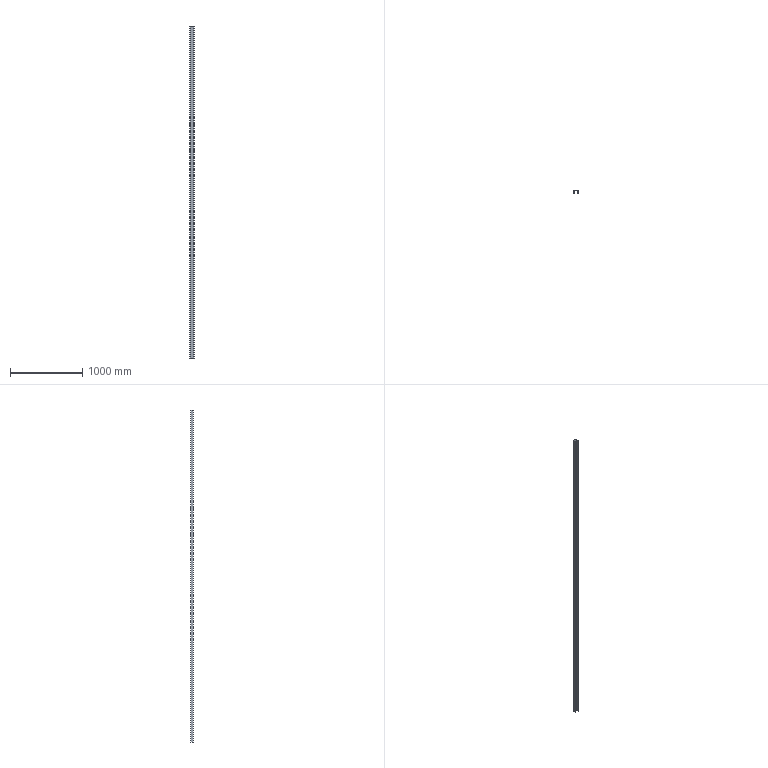Part | SolidWorks | features FlatPattern 1, SMBaseFlange 1, SheetMetal 1 | 1 solid | 22 faces | box 57 x 40 x 4600 mm | volume 1199908 mm3 | plane 18 | cylinder 4 | commonest cylinder face diameters 4 x2 8 x2
STEP:
#1=CARTESIAN_POINT('',(4.,0.,2300.));
#2=VERTEX_POINT('',#1);
#3=CARTESIAN_POINT('',(4.,-2.,2300.));
#4=VERTEX_POINT('',#3);
#5=CARTESIAN_POINT('',(4.,0.,2300.));
#6=DIRECTION('',(0.,-1.,0.));
#7=VECTOR('',#6,1000.);
#8=LINE('',#5,#7);
#9=EDGE_CURVE('',#2,#4,#8,.T.);
#10=ORIENTED_EDGE('',*,*,#9,.F.);
#11=CARTESIAN_POINT('',(0.,-4.,2300.));
#12=VERTEX_POINT('',#11);
#13=CARTESIAN_POINT('',(4.,-4.,2300.));
#14=DIRECTION('',(0.,0.,-1.));
#15=DIRECTION('',(1.,0.,0.));
#16=AXIS2_PLACEMENT_3D('',#13,#14,#15);
#17=CIRCLE('',#16,4.);
#18=EDGE_CURVE('',#12,#2,#17,.T.);
#19=ORIENTED_EDGE('',*,*,#18,.F.);
#20=CARTESIAN_POINT('',(2.,-4.,2300.));
#21=VERTEX_POINT('',#20);
#22=CARTESIAN_POINT('',(2.,-4.,2300.));
#23=DIRECTION('',(-1.,0.,0.));
#24=VECTOR('',#23,1000.);
#25=LINE('',#22,#24);
#26=EDGE_CURVE('',#21,#12,#25,.T.);
#27=ORIENTED_EDGE('',*,*,#26,.F.);
#28=CARTESIAN_POINT('',(4.,-4.,2300.));
#29=DIRECTION('',(0.,0.,-1.));
#30=DIRECTION('',(1.,0.,0.));
#31=AXIS2_PLACEMENT_3D('',#28,#29,#30);
#32=CIRCLE('',#31,2.);
#33=EDGE_CURVE('',#21,#4,#32,.T.);
#34=ORIENTED_EDGE('',*,*,#33,.T.);
#35=EDGE_LOOP('',(#10,#19,#27,#34));
#36=FACE_OUTER_BOUND('',#35,.T.);
#37=CARTESIAN_POINT('',(4.,0.,2300.));
#38=DIRECTION('',(0.,0.,1.));
#39=DIRECTION('',(1.,0.,0.));
#40=AXIS2_PLACEMENT_3D('',#37,#38,#39);
#41=PLANE('',#40);
#42=ADVANCED_FACE('',(#36),#41,.T.);
#43=CARTESIAN_POINT('',(53.,0.,2300.));
#44=VERTEX_POINT('',#43);
#45=CARTESIAN_POINT('',(57.,0.,2300.));
#46=DIRECTION('',(1.,0.,0.));
#47=VECTOR('',#46,1000.);
#48=LINE('',#45,#47);
#49=EDGE_CURVE('',#2,#44,#48,.T.);
#50=ORIENTED_EDGE('',*,*,#49,.F.);
#51=ORIENTED_EDGE('',*,*,#9,.T.);
#52=CARTESIAN_POINT('',(53.,-2.,2300.));
#53=VERTEX_POINT('',#52);
#54=CARTESIAN_POINT('',(57.,-2.,2300.));
#55=DIRECTION('',(1.,0.,0.));
#56=VECTOR('',#55,1000.);
#57=LINE('',#54,#56);
#58=EDGE_CURVE('',#4,#53,#57,.T.);
#59=ORIENTED_EDGE('',*,*,#58,.T.);
#60=CARTESIAN_POINT('',(53.,-2.,2300.));
#61=DIRECTION('',(0.,1.,0.));
#62=VECTOR('',#61,1000.);
#63=LINE('',#60,#62);
#64=EDGE_CURVE('',#53,#44,#63,.T.);
#65=ORIENTED_EDGE('',*,*,#64,.T.);
#66=EDGE_LOOP('',(#50,#51,#59,#65));
#67=FACE_OUTER_BOUND('',#66,.T.);
#68=CARTESIAN_POINT('',(2.,-4.,2300.));
#69=DIRECTION('',(0.,0.,1.));
#70=DIRECTION('',(1.,0.,0.));
#71=AXIS2_PLACEMENT_3D('',#68,#69,#70);
#72=PLANE('',#71);
#73=ADVANCED_FACE('',(#67),#72,.T.);
#74=CARTESIAN_POINT('',(0.,-4.,-2300.));
#75=VERTEX_POINT('',#74);
#76=CARTESIAN_POINT('',(2.,-4.,-2300.));
#77=VERTEX_POINT('',#76);
#78=CARTESIAN_POINT('',(0.,-4.,-2300.));
#79=DIRECTION('',(1.,0.,0.));
#80=VECTOR('',#79,1000.);
#81=LINE('',#78,#80);
#82=EDGE_CURVE('',#75,#77,#81,.T.);
#83=ORIENTED_EDGE('',*,*,#82,.F.);
#84=CARTESIAN_POINT('',(4.,0.,-2300.));
#85=VERTEX_POINT('',#84);
#86=CARTESIAN_POINT('',(4.,-4.,-2300.));
#87=DIRECTION('',(0.,0.,-1.));
#88=DIRECTION('',(1.,0.,0.));
#89=AXIS2_PLACEMENT_3D('',#86,#87,#88);
#90=CIRCLE('',#89,4.);
#91=EDGE_CURVE('',#75,#85,#90,.T.);
#92=ORIENTED_EDGE('',*,*,#91,.T.);
#93=CARTESIAN_POINT('',(4.,-2.,-2300.));
#94=VERTEX_POINT('',#93);
#95=CARTESIAN_POINT('',(4.,-2.,-2300.));
#96=DIRECTION('',(0.,1.,0.));
#97=VECTOR('',#96,1000.);
#98=LINE('',#95,#97);
#99=EDGE_CURVE('',#94,#85,#98,.T.);
#100=ORIENTED_EDGE('',*,*,#99,.F.);
#101=CARTESIAN_POINT('',(4.,-4.,-2300.));
#102=DIRECTION('',(0.,0.,-1.));
#103=DIRECTION('',(1.,0.,0.));
#104=AXIS2_PLACEMENT_3D('',#101,#102,#103);
#105=CIRCLE('',#104,2.);
#106=EDGE_CURVE('',#77,#94,#105,.T.);
#107=ORIENTED_EDGE('',*,*,#106,.F.);
#108=EDGE_LOOP('',(#83,#92,#100,#107));
#109=FACE_OUTER_BOUND('',#108,.T.);
#110=CARTESIAN_POINT('',(0.,-4.,-2300.));
#111=DIRECTION('',(0.,0.,-1.));
#112=DIRECTION('',(-1.,0.,0.));
#113=AXIS2_PLACEMENT_3D('',#110,#111,#112);
#114=PLANE('',#113);
#115=ADVANCED_FACE('',(#109),#114,.T.);
#116=CARTESIAN_POINT('',(0.,-40.,-2300.));
#117=VERTEX_POINT('',#116);
#118=CARTESIAN_POINT('',(0.,0.,-2300.));
#119=DIRECTION('',(0.,1.,0.));
#120=VECTOR('',#119,1000.);
#121=LINE('',#118,#120);
#122=EDGE_CURVE('',#117,#75,#121,.T.);
#123=ORIENTED_EDGE('',*,*,#122,.T.);
#124=ORIENTED_EDGE('',*,*,#82,.T.);
#125=CARTESIAN_POINT('',(2.,-40.,-2300.));
#126=VERTEX_POINT('',#125);
#127=CARTESIAN_POINT('',(2.,0.,-2300.));
#128=DIRECTION('',(0.,1.,0.));
#129=VECTOR('',#128,1000.);
#130=LINE('',#127,#129);
#131=EDGE_CURVE('',#126,#77,#130,.T.);
#132=ORIENTED_EDGE('',*,*,#131,.F.);
#133=CARTESIAN_POINT('',(2.,-40.,-2300.));
#134=DIRECTION('',(-1.,0.,0.));
#135=VECTOR('',#134,1000.);
#136=LINE('',#133,#135);
#137=EDGE_CURVE('',#126,#117,#136,.T.);
#138=ORIENTED_EDGE('',*,*,#137,.T.);
#139=EDGE_LOOP('',(#123,#124,#132,#138));
#140=FACE_OUTER_BOUND('',#139,.T.);
#141=CARTESIAN_POINT('',(4.,-2.,-2300.));
#142=DIRECTION('',(0.,0.,-1.));
#143=DIRECTION('',(-1.,0.,0.));
#144=AXIS2_PLACEMENT_3D('',#141,#142,#143);
#145=PLANE('',#144);
#146=ADVANCED_FACE('',(#140),#145,.T.);
#147=CARTESIAN_POINT('',(57.,-4.,2300.));
#148=VERTEX_POINT('',#147);
#149=CARTESIAN_POINT('',(55.,-4.,2300.));
#150=VERTEX_POINT('',#149);
#151=CARTESIAN_POINT('',(57.,-4.,2300.));
#152=DIRECTION('',(-1.,0.,0.));
#153=VECTOR('',#152,1000.);
#154=LINE('',#151,#153);
#155=EDGE_CURVE('',#148,#150,#154,.T.);
#156=ORIENTED_EDGE('',*,*,#155,.F.);
#157=CARTESIAN_POINT('',(53.,-4.,2300.));
#158=DIRECTION('',(0.,0.,-1.));
#159=DIRECTION('',(1.,0.,0.));
#160=AXIS2_PLACEMENT_3D('',#157,#158,#159);
#161=CIRCLE('',#160,4.);
#162=EDGE_CURVE('',#44,#148,#161,.T.);
#163=ORIENTED_EDGE('',*,*,#162,.F.);
#164=ORIENTED_EDGE('',*,*,#64,.F.);
#165=CARTESIAN_POINT('',(53.,-4.,2300.));
#166=DIRECTION('',(0.,0.,-1.));
#167=DIRECTION('',(1.,0.,0.));
#168=AXIS2_PLACEMENT_3D('',#165,#166,#167);
#169=CIRCLE('',#168,2.);
#170=EDGE_CURVE('',#53,#150,#169,.T.);
#171=ORIENTED_EDGE('',*,*,#170,.T.);
#172=EDGE_LOOP('',(#156,#163,#164,#171));
#173=FACE_OUTER_BOUND('',#172,.T.);
#174=CARTESIAN_POINT('',(57.,-4.,2300.));
#175=DIRECTION('',(0.,0.,1.));
#176=DIRECTION('',(1.,0.,0.));
#177=AXIS2_PLACEMENT_3D('',#174,#175,#176);
#178=PLANE('',#177);
#179=ADVANCED_FACE('',(#173),#178,.T.);
#180=CARTESIAN_POINT('',(57.,-40.,2300.));
#181=VERTEX_POINT('',#180);
#182=CARTESIAN_POINT('',(57.,0.,2300.));
#183=DIRECTION('',(0.,-1.,0.));
#184=VECTOR('',#183,1000.);
#185=LINE('',#182,#184);
#186=EDGE_CURVE('',#148,#181,#185,.T.);
#187=ORIENTED_EDGE('',*,*,#186,.F.);
#188=ORIENTED_EDGE('',*,*,#155,.T.);
#189=CARTESIAN_POINT('',(55.,-40.,2300.));
#190=VERTEX_POINT('',#189);
#191=CARTESIAN_POINT('',(55.,0.,2300.));
#192=DIRECTION('',(0.,-1.,0.));
#193=VECTOR('',#192,1000.);
#194=LINE('',#191,#193);
#195=EDGE_CURVE('',#150,#190,#194,.T.);
#196=ORIENTED_EDGE('',*,*,#195,.T.);
#197=CARTESIAN_POINT('',(57.,-40.,2300.));
#198=DIRECTION('',(-1.,0.,0.));
#199=VECTOR('',#198,1000.);
#200=LINE('',#197,#199);
#201=EDGE_CURVE('',#181,#190,#200,.T.);
#202=ORIENTED_EDGE('',*,*,#201,.F.);
#203=EDGE_LOOP('',(#187,#188,#196,#202));
#204=FACE_OUTER_BOUND('',#203,.T.);
#205=CARTESIAN_POINT('',(53.,-2.,2300.));
#206=DIRECTION('',(0.,0.,1.));
#207=DIRECTION('',(1.,0.,0.));
#208=AXIS2_PLACEMENT_3D('',#205,#206,#207);
#209=PLANE('',#208);
#210=ADVANCED_FACE('',(#204),#209,.T.);
#211=CARTESIAN_POINT('',(53.,0.,-2300.));
#212=VERTEX_POINT('',#211);
#213=CARTESIAN_POINT('',(53.,-2.,-2300.));
#214=VERTEX_POINT('',#213);
#215=CARTESIAN_POINT('',(53.,0.,-2300.));
#216=DIRECTION('',(0.,-1.,0.));
#217=VECTOR('',#216,1000.);
#218=LINE('',#215,#217);
#219=EDGE_CURVE('',#212,#214,#218,.T.);
#220=ORIENTED_EDGE('',*,*,#219,.F.);
#221=CARTESIAN_POINT('',(57.,-4.,-2300.));
#222=VERTEX_POINT('',#221);
#223=CARTESIAN_POINT('',(53.,-4.,-2300.));
#224=DIRECTION('',(0.,0.,-1.));
#225=DIRECTION('',(1.,0.,0.));
#226=AXIS2_PLACEMENT_3D('',#223,#224,#225);
#227=CIRCLE('',#226,4.);
#228=EDGE_CURVE('',#212,#222,#227,.T.);
#229=ORIENTED_EDGE('',*,*,#228,.T.);
#230=CARTESIAN_POINT('',(55.,-4.,-2300.));
#231=VERTEX_POINT('',#230);
#232=CARTESIAN_POINT('',(55.,-4.,-2300.));
#233=DIRECTION('',(1.,0.,0.));
#234=VECTOR('',#233,1000.);
#235=LINE('',#232,#234);
#236=EDGE_CURVE('',#231,#222,#235,.T.);
#237=ORIENTED_EDGE('',*,*,#236,.F.);
#238=CARTESIAN_POINT('',(53.,-4.,-2300.));
#239=DIRECTION('',(0.,0.,-1.));
#240=DIRECTION('',(1.,0.,0.));
#241=AXIS2_PLACEMENT_3D('',#238,#239,#240);
#242=CIRCLE('',#241,2.);
#243=EDGE_CURVE('',#214,#231,#242,.T.);
#244=ORIENTED_EDGE('',*,*,#243,.F.);
#245=EDGE_LOOP('',(#220,#229,#237,#244));
#246=FACE_OUTER_BOUND('',#245,.T.);
#247=CARTESIAN_POINT('',(53.,0.,-2300.));
#248=DIRECTION('',(0.,0.,-1.));
#249=DIRECTION('',(-1.,0.,0.));
#250=AXIS2_PLACEMENT_3D('',#247,#248,#249);
#251=PLANE('',#250);
#252=ADVANCED_FACE('',(#246),#251,.T.);
#253=CARTESIAN_POINT('',(57.,0.,-2300.));
#254=DIRECTION('',(1.,0.,0.));
#255=VECTOR('',#254,1000.);
#256=LINE('',#253,#255);
#257=EDGE_CURVE('',#85,#212,#256,.T.);
#258=ORIENTED_EDGE('',*,*,#257,.T.);
#259=ORIENTED_EDGE('',*,*,#219,.T.);
#260=CARTESIAN_POINT('',(57.,-2.,-2300.));
#261=DIRECTION('',(1.,0.,0.));
#262=VECTOR('',#261,1000.);
#263=LINE('',#260,#262);
#264=EDGE_CURVE('',#94,#214,#263,.T.);
#265=ORIENTED_EDGE('',*,*,#264,.F.);
#266=ORIENTED_EDGE('',*,*,#99,.T.);
#267=EDGE_LOOP('',(#258,#259,#265,#266));
#268=FACE_OUTER_BOUND('',#267,.T.);
#269=CARTESIAN_POINT('',(55.,-4.,-2300.));
#270=DIRECTION('',(0.,0.,-1.));
#271=DIRECTION('',(-1.,0.,0.));
#272=AXIS2_PLACEMENT_3D('',#269,#270,#271);
#273=PLANE('',#272);
#274=ADVANCED_FACE('',(#268),#273,.T.);
#275=CARTESIAN_POINT('',(55.,-40.,-2300.));
#276=VERTEX_POINT('',#275);
#277=CARTESIAN_POINT('',(55.,0.,-2300.));
#278=DIRECTION('',(0.,-1.,0.));
#279=VECTOR('',#278,1000.);
#280=LINE('',#277,#279);
#281=EDGE_CURVE('',#231,#276,#280,.T.);
#282=ORIENTED_EDGE('',*,*,#281,.T.);
#283=CARTESIAN_POINT('',(55.,-40.,2300.));
#284=DIRECTION('',(0.,0.,-1.));
#285=VECTOR('',#284,1000.);
#286=LINE('',#283,#285);
#287=EDGE_CURVE('',#190,#276,#286,.T.);
#288=ORIENTED_EDGE('',*,*,#287,.F.);
#289=ORIENTED_EDGE('',*,*,#195,.F.);
#290=CARTESIAN_POINT('',(55.,-4.,2300.));
#291=DIRECTION('',(0.,0.,-1.));
#292=VECTOR('',#291,1000.);
#293=LINE('',#290,#292);
#294=EDGE_CURVE('',#150,#231,#293,.T.);
#295=ORIENTED_EDGE('',*,*,#294,.T.);
#296=EDGE_LOOP('',(#282,#288,#289,#295));
#297=FACE_OUTER_BOUND('',#296,.T.);
#298=CARTESIAN_POINT('',(55.,0.,2300.));
#299=DIRECTION('',(1.,0.,0.));
#300=DIRECTION('',(0.,0.,-1.));
#301=AXIS2_PLACEMENT_3D('',#298,#299,#300);
#302=PLANE('',#301);
#303=ADVANCED_FACE('',(#297),#302,.F.);
#304=CARTESIAN_POINT('',(57.,-40.,-2300.));
#305=VERTEX_POINT('',#304);
#306=CARTESIAN_POINT('',(57.,-40.,-2300.));
#307=DIRECTION('',(-1.,0.,0.));
#308=VECTOR('',#307,1000.);
#309=LINE('',#306,#308);
#310=EDGE_CURVE('',#305,#276,#309,.T.);
#311=ORIENTED_EDGE('',*,*,#310,.F.);
#312=CARTESIAN_POINT('',(57.,-40.,2300.));
#313=DIRECTION('',(0.,0.,-1.));
#314=VECTOR('',#313,1000.);
#315=LINE('',#312,#314);
#316=EDGE_CURVE('',#181,#305,#315,.T.);
#317=ORIENTED_EDGE('',*,*,#316,.F.);
#318=ORIENTED_EDGE('',*,*,#201,.T.);
#319=ORIENTED_EDGE('',*,*,#287,.T.);
#320=EDGE_LOOP('',(#311,#317,#318,#319));
#321=FACE_OUTER_BOUND('',#320,.T.);
#322=CARTESIAN_POINT('',(57.,-40.,2300.));
#323=DIRECTION('',(0.,-1.,0.));
#324=DIRECTION('',(0.,0.,-1.));
#325=AXIS2_PLACEMENT_3D('',#322,#323,#324);
#326=PLANE('',#325);
#327=ADVANCED_FACE('',(#321),#326,.T.);
#328=CARTESIAN_POINT('',(57.,0.,-2300.));
#329=DIRECTION('',(0.,-1.,0.));
#330=VECTOR('',#329,1000.);
#331=LINE('',#328,#330);
#332=EDGE_CURVE('',#222,#305,#331,.T.);
#333=ORIENTED_EDGE('',*,*,#332,.F.);
#334=CARTESIAN_POINT('',(57.,-4.,2300.));
#335=DIRECTION('',(0.,0.,-1.));
#336=VECTOR('',#335,1000.);
#337=LINE('',#334,#336);
#338=EDGE_CURVE('',#148,#222,#337,.T.);
#339=ORIENTED_EDGE('',*,*,#338,.F.);
#340=ORIENTED_EDGE('',*,*,#186,.T.);
#341=ORIENTED_EDGE('',*,*,#316,.T.);
#342=EDGE_LOOP('',(#333,#339,#340,#341));
#343=FACE_OUTER_BOUND('',#342,.T.);
#344=CARTESIAN_POINT('',(57.,0.,2300.));
#345=DIRECTION('',(1.,0.,0.));
#346=DIRECTION('',(0.,0.,-1.));
#347=AXIS2_PLACEMENT_3D('',#344,#345,#346);
#348=PLANE('',#347);
#349=ADVANCED_FACE('',(#343),#348,.T.);
#350=ORIENTED_EDGE('',*,*,#228,.F.);
#351=CARTESIAN_POINT('',(53.,0.,2300.));
#352=DIRECTION('',(0.,0.,-1.));
#353=VECTOR('',#352,1000.);
#354=LINE('',#351,#353);
#355=EDGE_CURVE('',#44,#212,#354,.T.);
#356=ORIENTED_EDGE('',*,*,#355,.F.);
#357=ORIENTED_EDGE('',*,*,#162,.T.);
#358=ORIENTED_EDGE('',*,*,#338,.T.);
#359=EDGE_LOOP('',(#350,#356,#357,#358));
#360=FACE_OUTER_BOUND('',#359,.T.);
#361=CARTESIAN_POINT('',(53.,-4.,2300.));
#362=DIRECTION('',(0.,0.,-1.));
#363=DIRECTION('',(-1.,0.,0.));
#364=AXIS2_PLACEMENT_3D('',#361,#362,#363);
#365=CYLINDRICAL_SURFACE('',#364,4.);
#366=ADVANCED_FACE('',(#360),#365,.T.);
#367=ORIENTED_EDGE('',*,*,#257,.F.);
#368=CARTESIAN_POINT('',(4.,0.,2300.));
#369=DIRECTION('',(0.,0.,-1.));
#370=VECTOR('',#369,1000.);
#371=LINE('',#368,#370);
#372=EDGE_CURVE('',#2,#85,#371,.T.);
#373=ORIENTED_EDGE('',*,*,#372,.F.);
#374=ORIENTED_EDGE('',*,*,#49,.T.);
#375=ORIENTED_EDGE('',*,*,#355,.T.);
#376=EDGE_LOOP('',(#367,#373,#374,#375));
#377=FACE_OUTER_BOUND('',#376,.T.);
#378=CARTESIAN_POINT('',(57.,0.,2300.));
#379=DIRECTION('',(0.,1.,0.));
#380=DIRECTION('',(0.,0.,1.));
#381=AXIS2_PLACEMENT_3D('',#378,#379,#380);
#382=PLANE('',#381);
#383=ADVANCED_FACE('',(#377),#382,.T.);
#384=ORIENTED_EDGE('',*,*,#91,.F.);
#385=CARTESIAN_POINT('',(0.,-4.,2300.));
#386=DIRECTION('',(0.,0.,-1.));
#387=VECTOR('',#386,1000.);
#388=LINE('',#385,#387);
#389=EDGE_CURVE('',#12,#75,#388,.T.);
#390=ORIENTED_EDGE('',*,*,#389,.F.);
#391=ORIENTED_EDGE('',*,*,#18,.T.);
#392=ORIENTED_EDGE('',*,*,#372,.T.);
#393=EDGE_LOOP('',(#384,#390,#391,#392));
#394=FACE_OUTER_BOUND('',#393,.T.);
#395=CARTESIAN_POINT('',(4.,-4.,2300.));
#396=DIRECTION('',(0.,0.,-1.));
#397=DIRECTION('',(-1.,0.,0.));
#398=AXIS2_PLACEMENT_3D('',#395,#396,#397);
#399=CYLINDRICAL_SURFACE('',#398,4.);
#400=ADVANCED_FACE('',(#394),#399,.T.);
#401=ORIENTED_EDGE('',*,*,#122,.F.);
#402=CARTESIAN_POINT('',(0.,-40.,2300.));
#403=VERTEX_POINT('',#402);
#404=CARTESIAN_POINT('',(0.,-40.,2300.));
#405=DIRECTION('',(0.,0.,-1.));
#406=VECTOR('',#405,1000.);
#407=LINE('',#404,#406);
#408=EDGE_CURVE('',#403,#117,#407,.T.);
#409=ORIENTED_EDGE('',*,*,#408,.F.);
#410=CARTESIAN_POINT('',(0.,0.,2300.));
#411=DIRECTION('',(0.,1.,0.));
#412=VECTOR('',#411,1000.);
#413=LINE('',#410,#412);
#414=EDGE_CURVE('',#403,#12,#413,.T.);
#415=ORIENTED_EDGE('',*,*,#414,.T.);
#416=ORIENTED_EDGE('',*,*,#389,.T.);
#417=EDGE_LOOP('',(#401,#409,#415,#416));
#418=FACE_OUTER_BOUND('',#417,.T.);
#419=CARTESIAN_POINT('',(0.,0.,2300.));
#420=DIRECTION('',(-1.,0.,0.));
#421=DIRECTION('',(0.,-1.,0.));
#422=AXIS2_PLACEMENT_3D('',#419,#420,#421);
#423=PLANE('',#422);
#424=ADVANCED_FACE('',(#418),#423,.T.);
#425=ORIENTED_EDGE('',*,*,#137,.F.);
#426=CARTESIAN_POINT('',(2.,-40.,2300.));
#427=VERTEX_POINT('',#426);
#428=CARTESIAN_POINT('',(2.,-40.,2300.));
#429=DIRECTION('',(0.,0.,-1.));
#430=VECTOR('',#429,1000.);
#431=LINE('',#428,#430);
#432=EDGE_CURVE('',#427,#126,#431,.T.);
#433=ORIENTED_EDGE('',*,*,#432,.F.);
#434=CARTESIAN_POINT('',(2.,-40.,2300.));
#435=DIRECTION('',(-1.,0.,0.));
#436=VECTOR('',#435,1000.);
#437=LINE('',#434,#436);
#438=EDGE_CURVE('',#427,#403,#437,.T.);
#439=ORIENTED_EDGE('',*,*,#438,.T.);
#440=ORIENTED_EDGE('',*,*,#408,.T.);
#441=EDGE_LOOP('',(#425,#433,#439,#440));
#442=FACE_OUTER_BOUND('',#441,.T.);
#443=CARTESIAN_POINT('',(2.,-40.,2300.));
#444=DIRECTION('',(0.,-1.,0.));
#445=DIRECTION('',(0.,0.,-1.));
#446=AXIS2_PLACEMENT_3D('',#443,#444,#445);
#447=PLANE('',#446);
#448=ADVANCED_FACE('',(#442),#447,.T.);
#449=ORIENTED_EDGE('',*,*,#131,.T.);
#450=CARTESIAN_POINT('',(2.,-4.,2300.));
#451=DIRECTION('',(0.,0.,-1.));
#452=VECTOR('',#451,1000.);
#453=LINE('',#450,#452);
#454=EDGE_CURVE('',#21,#77,#453,.T.);
#455=ORIENTED_EDGE('',*,*,#454,.F.);
#456=CARTESIAN_POINT('',(2.,0.,2300.));
#457=DIRECTION('',(0.,1.,0.));
#458=VECTOR('',#457,1000.);
#459=LINE('',#456,#458);
#460=EDGE_CURVE('',#427,#21,#459,.T.);
#461=ORIENTED_EDGE('',*,*,#460,.F.);
#462=ORIENTED_EDGE('',*,*,#432,.T.);
#463=EDGE_LOOP('',(#449,#455,#461,#462));
#464=FACE_OUTER_BOUND('',#463,.T.);
#465=CARTESIAN_POINT('',(2.,0.,2300.));
#466=DIRECTION('',(-1.,0.,0.));
#467=DIRECTION('',(0.,-1.,0.));
#468=AXIS2_PLACEMENT_3D('',#465,#466,#467);
#469=PLANE('',#468);
#470=ADVANCED_FACE('',(#464),#469,.F.);
#471=ORIENTED_EDGE('',*,*,#106,.T.);
#472=CARTESIAN_POINT('',(4.,-2.,2300.));
#473=DIRECTION('',(0.,0.,-1.));
#474=VECTOR('',#473,1000.);
#475=LINE('',#472,#474);
#476=EDGE_CURVE('',#4,#94,#475,.T.);
#477=ORIENTED_EDGE('',*,*,#476,.F.);
#478=ORIENTED_EDGE('',*,*,#33,.F.);
#479=ORIENTED_EDGE('',*,*,#454,.T.);
#480=EDGE_LOOP('',(#471,#477,#478,#479));
#481=FACE_OUTER_BOUND('',#480,.T.);
#482=CARTESIAN_POINT('',(4.,-4.,2300.));
#483=DIRECTION('',(0.,0.,-1.));
#484=DIRECTION('',(-1.,0.,0.));
#485=AXIS2_PLACEMENT_3D('',#482,#483,#484);
#486=CYLINDRICAL_SURFACE('',#485,2.);
#487=ADVANCED_FACE('',(#481),#486,.F.);
#488=ORIENTED_EDGE('',*,*,#264,.T.);
#489=CARTESIAN_POINT('',(53.,-2.,2300.));
#490=DIRECTION('',(0.,0.,-1.));
#491=VECTOR('',#490,1000.);
#492=LINE('',#489,#491);
#493=EDGE_CURVE('',#53,#214,#492,.T.);
#494=ORIENTED_EDGE('',*,*,#493,.F.);
#495=ORIENTED_EDGE('',*,*,#58,.F.);
#496=ORIENTED_EDGE('',*,*,#476,.T.);
#497=EDGE_LOOP('',(#488,#494,#495,#496));
#498=FACE_OUTER_BOUND('',#497,.T.);
#499=CARTESIAN_POINT('',(57.,-2.,2300.));
#500=DIRECTION('',(0.,1.,0.));
#501=DIRECTION('',(0.,0.,1.));
#502=AXIS2_PLACEMENT_3D('',#499,#500,#501);
#503=PLANE('',#502);
#504=ADVANCED_FACE('',(#498),#503,.F.);
#505=ORIENTED_EDGE('',*,*,#243,.T.);
#506=ORIENTED_EDGE('',*,*,#294,.F.);
#507=ORIENTED_EDGE('',*,*,#170,.F.);
#508=ORIENTED_EDGE('',*,*,#493,.T.);
#509=EDGE_LOOP('',(#505,#506,#507,#508));
#510=FACE_OUTER_BOUND('',#509,.T.);
#511=CARTESIAN_POINT('',(53.,-4.,2300.));
#512=DIRECTION('',(0.,0.,-1.));
#513=DIRECTION('',(-1.,0.,0.));
#514=AXIS2_PLACEMENT_3D('',#511,#512,#513);
#515=CYLINDRICAL_SURFACE('',#514,2.);
#516=ADVANCED_FACE('',(#510),#515,.F.);
#517=ORIENTED_EDGE('',*,*,#460,.T.);
#518=ORIENTED_EDGE('',*,*,#26,.T.);
#519=ORIENTED_EDGE('',*,*,#414,.F.);
#520=ORIENTED_EDGE('',*,*,#438,.F.);
#521=EDGE_LOOP('',(#517,#518,#519,#520));
#522=FACE_OUTER_BOUND('',#521,.T.);
#523=CARTESIAN_POINT('',(53.,-4.,2300.));
#524=DIRECTION('',(0.,0.,1.));
#525=DIRECTION('',(1.,0.,0.));
#526=AXIS2_PLACEMENT_3D('',#523,#524,#525);
#527=PLANE('',#526);
#528=ADVANCED_FACE('',(#522),#527,.T.);
#529=ORIENTED_EDGE('',*,*,#281,.F.);
#530=ORIENTED_EDGE('',*,*,#236,.T.);
#531=ORIENTED_EDGE('',*,*,#332,.T.);
#532=ORIENTED_EDGE('',*,*,#310,.T.);
#533=EDGE_LOOP('',(#529,#530,#531,#532));
#534=FACE_OUTER_BOUND('',#533,.T.);
#535=CARTESIAN_POINT('',(53.,-4.,-2300.));
#536=DIRECTION('',(0.,0.,1.));
#537=DIRECTION('',(1.,0.,0.));
#538=AXIS2_PLACEMENT_3D('',#535,#536,#537);
#539=PLANE('',#538);
#540=ADVANCED_FACE('',(#534),#539,.F.);
#541=CLOSED_SHELL('',(#42,#73,#115,#146,#179,#210,#252,#274,#303,#327,#349,#366,#383,#400,#424,#448,#470,#487,#504,#516,#528,#540));
#542=MANIFOLD_SOLID_BREP('',#541);
#543=CARTESIAN_POINT('',(0.,0.,0.));
#544=DIRECTION('',(0.,0.,1.));
#545=DIRECTION('',(1.,0.,0.));
#546=AXIS2_PLACEMENT_3D('',#543,#544,#545);
#547=(LENGTH_UNIT()NAMED_UNIT(*)SI_UNIT(.MILLI.,.METRE.));
#548=UNCERTAINTY_MEASURE_WITH_UNIT(LENGTH_MEASURE(0.00001),#547,'','');
#549=(NAMED_UNIT(*)PLANE_ANGLE_UNIT()SI_UNIT($,.RADIAN.));
#550=(NAMED_UNIT(*)SI_UNIT($,.STERADIAN.)SOLID_ANGLE_UNIT());
#551=(GEOMETRIC_REPRESENTATION_CONTEXT(3)GLOBAL_UNCERTAINTY_ASSIGNED_CONTEXT((#548))GLOBAL_UNIT_ASSIGNED_CONTEXT((#547,#549,#550))REPRESENTATION_CONTEXT('',''));
#552=ADVANCED_BREP_SHAPE_REPRESENTATION('',(#542,#546),#551);